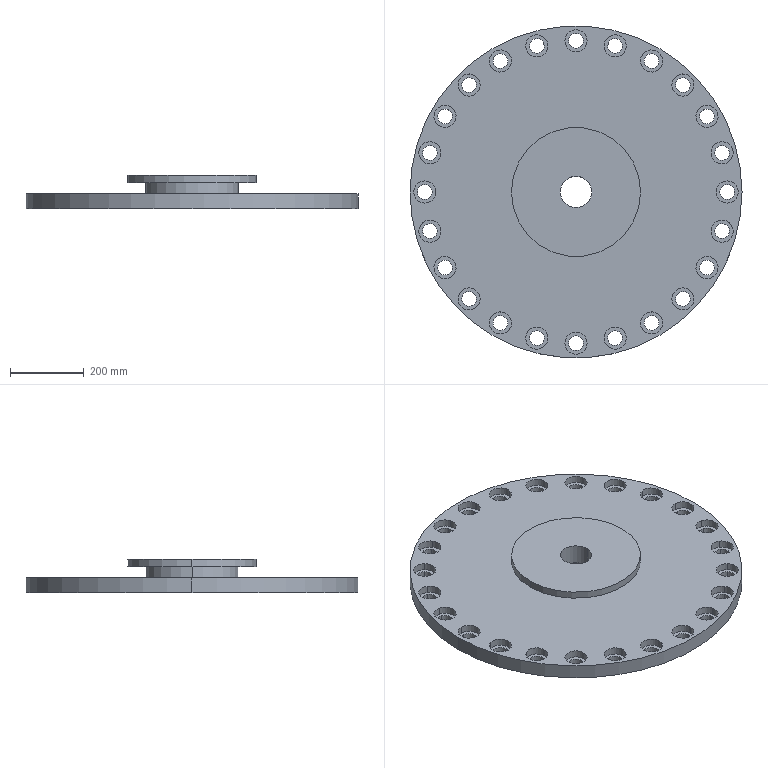Part | SolidWorks | features ICE 3, CirPattern 1, Extrusion 1, HoleWzd 1 | 1 solid | 135 faces | box 900 x 900 x 90 mm | volume 25700427 mm3 | cylinder 106 | plane 29 | commonest cylinder face diameters 40 x48 60 x48 85 x2 180 x2 250 x2 350 x2